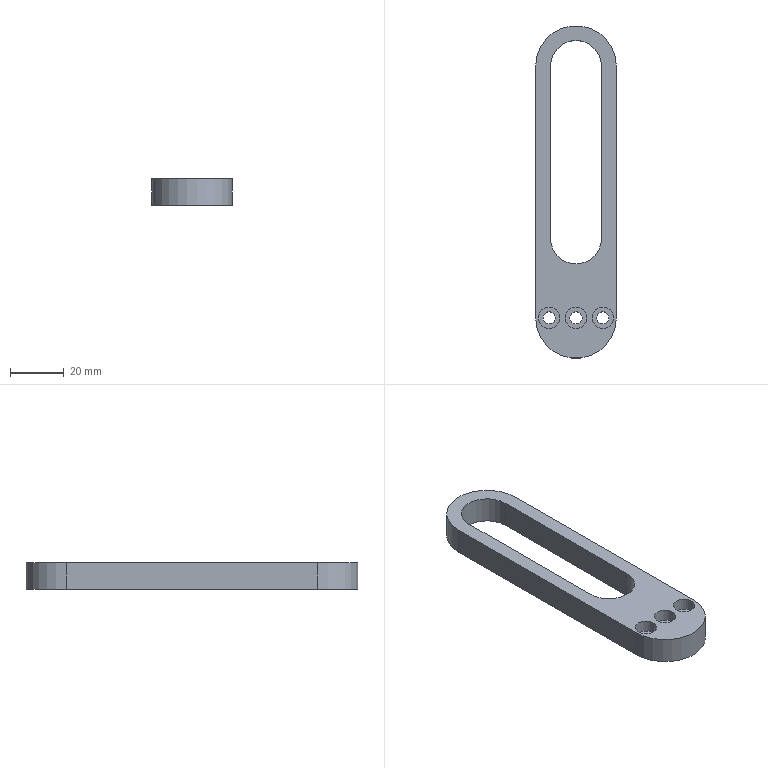Part | STEP file | 1 solid | 21 faces | box 30 x 123.5 x 10 mm | volume 18320 mm3 | cylinder 11 | plane 10 | commonest cylinder face diameters 4.5 x3 8 x3 19 x2 30 x2 28 x1
STEP:
#1=CARTESIAN_POINT('',(0.,0.,0.));
#2=DIRECTION('',(0.,0.,1.));
#3=DIRECTION('',(1.,0.,0.));
#4=AXIS2_PLACEMENT_3D('',#1,#2,#3);
#5=CARTESIAN_POINT('',(9.5,44.5,0.));
#6=VERTEX_POINT('',#5);
#7=CARTESIAN_POINT('',(9.5,108.5,0.));
#8=VERTEX_POINT('',#7);
#9=CARTESIAN_POINT('',(9.5,44.5,0.));
#10=DIRECTION('',(0.,1.,0.));
#11=VECTOR('',#10,1.);
#12=LINE('',#9,#11);
#13=CARTESIAN_POINT('',(9.5,44.5,0.));
#14=DIRECTION('',(-1.,0.,0.));
#15=DIRECTION('',(0.,0.,1.));
#16=AXIS2_PLACEMENT_3D('',#13,#14,#15);
#17=PLANE('',#16);
#18=CARTESIAN_POINT('',(0.,0.));
#19=DIRECTION('',(0.,1.));
#20=VECTOR('',#19,1.);
#21=LINE('',#18,#20);
#22=(GEOMETRIC_REPRESENTATION_CONTEXT(2)PARAMETRIC_REPRESENTATION_CONTEXT()REPRESENTATION_CONTEXT('',''));
#23=DEFINITIONAL_REPRESENTATION('',(#21),#22);
#24=PCURVE('',#17,#23);
#25=CARTESIAN_POINT('',(0.,0.,0.));
#26=DIRECTION('',(0.,0.,1.));
#27=DIRECTION('',(1.,0.,0.));
#28=AXIS2_PLACEMENT_3D('',#25,#26,#27);
#29=PLANE('',#28);
#30=CARTESIAN_POINT('',(9.5,44.5));
#31=DIRECTION('',(0.,1.));
#32=VECTOR('',#31,1.);
#33=LINE('',#30,#32);
#34=(GEOMETRIC_REPRESENTATION_CONTEXT(2)PARAMETRIC_REPRESENTATION_CONTEXT()REPRESENTATION_CONTEXT('',''));
#35=DEFINITIONAL_REPRESENTATION('',(#33),#34);
#36=PCURVE('',#29,#35);
#37=SURFACE_CURVE('',#12,(#24,#36),.PCURVE_S1.);
#38=EDGE_CURVE('',#6,#8,#37,.T.);
#39=ORIENTED_EDGE('',*,*,#38,.F.);
#40=CARTESIAN_POINT('',(9.5,44.5,10.));
#41=VERTEX_POINT('',#40);
#42=CARTESIAN_POINT('',(9.5,44.5,0.));
#43=DIRECTION('',(0.,0.,1.));
#44=VECTOR('',#43,1.);
#45=LINE('',#42,#44);
#46=CARTESIAN_POINT('',(0.,0.));
#47=DIRECTION('',(1.,0.));
#48=VECTOR('',#47,1.);
#49=LINE('',#46,#48);
#50=(GEOMETRIC_REPRESENTATION_CONTEXT(2)PARAMETRIC_REPRESENTATION_CONTEXT()REPRESENTATION_CONTEXT('',''));
#51=DEFINITIONAL_REPRESENTATION('',(#49),#50);
#52=PCURVE('',#17,#51);
#53=CARTESIAN_POINT('',(0.,44.5,0.));
#54=DIRECTION('',(0.,0.,1.));
#55=DIRECTION('',(-1.,0.,0.));
#56=AXIS2_PLACEMENT_3D('',#53,#54,#55);
#57=CYLINDRICAL_SURFACE('',#56,9.5);
#58=CARTESIAN_POINT('',(3.142,0.));
#59=DIRECTION('',(0.,1.));
#60=VECTOR('',#59,1.);
#61=LINE('',#58,#60);
#62=(GEOMETRIC_REPRESENTATION_CONTEXT(2)PARAMETRIC_REPRESENTATION_CONTEXT()REPRESENTATION_CONTEXT('',''));
#63=DEFINITIONAL_REPRESENTATION('',(#61),#62);
#64=PCURVE('',#57,#63);
#65=SURFACE_CURVE('',#45,(#52,#64),.PCURVE_S1.);
#66=EDGE_CURVE('',#6,#41,#65,.T.);
#67=ORIENTED_EDGE('',*,*,#66,.T.);
#68=CARTESIAN_POINT('',(9.5,108.5,10.));
#69=VERTEX_POINT('',#68);
#70=CARTESIAN_POINT('',(9.5,44.5,10.));
#71=DIRECTION('',(0.,1.,0.));
#72=VECTOR('',#71,1.);
#73=LINE('',#70,#72);
#74=CARTESIAN_POINT('',(10.,0.));
#75=DIRECTION('',(0.,1.));
#76=VECTOR('',#75,1.);
#77=LINE('',#74,#76);
#78=(GEOMETRIC_REPRESENTATION_CONTEXT(2)PARAMETRIC_REPRESENTATION_CONTEXT()REPRESENTATION_CONTEXT('',''));
#79=DEFINITIONAL_REPRESENTATION('',(#77),#78);
#80=PCURVE('',#17,#79);
#81=CARTESIAN_POINT('',(0.,0.,10.));
#82=DIRECTION('',(0.,0.,1.));
#83=DIRECTION('',(1.,0.,0.));
#84=AXIS2_PLACEMENT_3D('',#81,#82,#83);
#85=PLANE('',#84);
#86=CARTESIAN_POINT('',(9.5,44.5));
#87=DIRECTION('',(0.,1.));
#88=VECTOR('',#87,1.);
#89=LINE('',#86,#88);
#90=(GEOMETRIC_REPRESENTATION_CONTEXT(2)PARAMETRIC_REPRESENTATION_CONTEXT()REPRESENTATION_CONTEXT('',''));
#91=DEFINITIONAL_REPRESENTATION('',(#89),#90);
#92=PCURVE('',#85,#91);
#93=SURFACE_CURVE('',#73,(#80,#92),.PCURVE_S1.);
#94=EDGE_CURVE('',#41,#69,#93,.T.);
#95=ORIENTED_EDGE('',*,*,#94,.T.);
#96=CARTESIAN_POINT('',(9.5,108.5,0.));
#97=DIRECTION('',(0.,0.,1.));
#98=VECTOR('',#97,1.);
#99=LINE('',#96,#98);
#100=CARTESIAN_POINT('',(0.,64.));
#101=DIRECTION('',(1.,0.));
#102=VECTOR('',#101,1.);
#103=LINE('',#100,#102);
#104=(GEOMETRIC_REPRESENTATION_CONTEXT(2)PARAMETRIC_REPRESENTATION_CONTEXT()REPRESENTATION_CONTEXT('',''));
#105=DEFINITIONAL_REPRESENTATION('',(#103),#104);
#106=PCURVE('',#17,#105);
#107=CARTESIAN_POINT('',(0.,108.5,0.));
#108=DIRECTION('',(0.,0.,1.));
#109=DIRECTION('',(1.,0.,0.));
#110=AXIS2_PLACEMENT_3D('',#107,#108,#109);
#111=CYLINDRICAL_SURFACE('',#110,9.5);
#112=CARTESIAN_POINT('',(0.,0.));
#113=DIRECTION('',(0.,1.));
#114=VECTOR('',#113,1.);
#115=LINE('',#112,#114);
#116=(GEOMETRIC_REPRESENTATION_CONTEXT(2)PARAMETRIC_REPRESENTATION_CONTEXT()REPRESENTATION_CONTEXT('',''));
#117=DEFINITIONAL_REPRESENTATION('',(#115),#116);
#118=PCURVE('',#111,#117);
#119=SURFACE_CURVE('',#99,(#106,#118),.PCURVE_S1.);
#120=EDGE_CURVE('',#8,#69,#119,.T.);
#121=ORIENTED_EDGE('',*,*,#120,.F.);
#122=EDGE_LOOP('',(#39,#67,#95,#121));
#123=FACE_BOUND('',#122,.T.);
#124=ADVANCED_FACE('',(#123),#17,.T.);
#125=CARTESIAN_POINT('',(-15.,108.5,0.));
#126=VERTEX_POINT('',#125);
#127=CARTESIAN_POINT('',(-15.,15.,0.));
#128=VERTEX_POINT('',#127);
#129=CARTESIAN_POINT('',(-15.,108.5,0.));
#130=DIRECTION('',(0.,-1.,0.));
#131=VECTOR('',#130,1.);
#132=LINE('',#129,#131);
#133=CARTESIAN_POINT('',(-15.,108.5));
#134=DIRECTION('',(0.,-1.));
#135=VECTOR('',#134,1.);
#136=LINE('',#133,#135);
#137=(GEOMETRIC_REPRESENTATION_CONTEXT(2)PARAMETRIC_REPRESENTATION_CONTEXT()REPRESENTATION_CONTEXT('',''));
#138=DEFINITIONAL_REPRESENTATION('',(#136),#137);
#139=PCURVE('',#29,#138);
#140=CARTESIAN_POINT('',(-15.,15.,0.));
#141=DIRECTION('',(-1.,0.,0.));
#142=DIRECTION('',(0.,0.,1.));
#143=AXIS2_PLACEMENT_3D('',#140,#141,#142);
#144=PLANE('',#143);
#145=CARTESIAN_POINT('',(0.,93.5));
#146=DIRECTION('',(0.,-1.));
#147=VECTOR('',#146,1.);
#148=LINE('',#145,#147);
#149=(GEOMETRIC_REPRESENTATION_CONTEXT(2)PARAMETRIC_REPRESENTATION_CONTEXT()REPRESENTATION_CONTEXT('',''));
#150=DEFINITIONAL_REPRESENTATION('',(#148),#149);
#151=PCURVE('',#144,#150);
#152=SURFACE_CURVE('',#132,(#139,#151),.PCURVE_S1.);
#153=EDGE_CURVE('',#126,#128,#152,.T.);
#154=ORIENTED_EDGE('',*,*,#153,.F.);
#155=CARTESIAN_POINT('',(15.,108.5,0.));
#156=VERTEX_POINT('',#155);
#157=CARTESIAN_POINT('',(0.,108.5,0.));
#158=DIRECTION('',(0.,0.,1.));
#159=DIRECTION('',(1.,0.,0.));
#160=AXIS2_PLACEMENT_3D('',#157,#158,#159);
#161=CIRCLE('',#160,15.);
#162=CARTESIAN_POINT('',(0.,108.5));
#163=DIRECTION('',(1.,0.));
#164=AXIS2_PLACEMENT_2D('',#162,#163);
#165=CIRCLE('',#164,15.);
#166=(GEOMETRIC_REPRESENTATION_CONTEXT(2)PARAMETRIC_REPRESENTATION_CONTEXT()REPRESENTATION_CONTEXT('',''));
#167=DEFINITIONAL_REPRESENTATION('',(#165),#166);
#168=PCURVE('',#29,#167);
#169=CARTESIAN_POINT('',(0.,108.5,0.));
#170=DIRECTION('',(0.,0.,1.));
#171=DIRECTION('',(1.,0.,0.));
#172=AXIS2_PLACEMENT_3D('',#169,#170,#171);
#173=CYLINDRICAL_SURFACE('',#172,15.);
#174=CARTESIAN_POINT('',(0.,0.));
#175=DIRECTION('',(1.,0.));
#176=VECTOR('',#175,1.);
#177=LINE('',#174,#176);
#178=(GEOMETRIC_REPRESENTATION_CONTEXT(2)PARAMETRIC_REPRESENTATION_CONTEXT()REPRESENTATION_CONTEXT('',''));
#179=DEFINITIONAL_REPRESENTATION('',(#177),#178);
#180=PCURVE('',#173,#179);
#181=SURFACE_CURVE('',#161,(#168,#180),.PCURVE_S1.);
#182=EDGE_CURVE('',#156,#126,#181,.T.);
#183=ORIENTED_EDGE('',*,*,#182,.F.);
#184=CARTESIAN_POINT('',(15.,15.,0.));
#185=VERTEX_POINT('',#184);
#186=CARTESIAN_POINT('',(15.,15.,0.));
#187=DIRECTION('',(0.,1.,0.));
#188=VECTOR('',#187,1.);
#189=LINE('',#186,#188);
#190=CARTESIAN_POINT('',(15.,15.));
#191=DIRECTION('',(0.,1.));
#192=VECTOR('',#191,1.);
#193=LINE('',#190,#192);
#194=(GEOMETRIC_REPRESENTATION_CONTEXT(2)PARAMETRIC_REPRESENTATION_CONTEXT()REPRESENTATION_CONTEXT('',''));
#195=DEFINITIONAL_REPRESENTATION('',(#193),#194);
#196=PCURVE('',#29,#195);
#197=CARTESIAN_POINT('',(15.,108.5,0.));
#198=DIRECTION('',(1.,0.,0.));
#199=DIRECTION('',(0.,0.,-1.));
#200=AXIS2_PLACEMENT_3D('',#197,#198,#199);
#201=PLANE('',#200);
#202=CARTESIAN_POINT('',(0.,-93.5));
#203=DIRECTION('',(0.,1.));
#204=VECTOR('',#203,1.);
#205=LINE('',#202,#204);
#206=(GEOMETRIC_REPRESENTATION_CONTEXT(2)PARAMETRIC_REPRESENTATION_CONTEXT()REPRESENTATION_CONTEXT('',''));
#207=DEFINITIONAL_REPRESENTATION('',(#205),#206);
#208=PCURVE('',#201,#207);
#209=SURFACE_CURVE('',#189,(#196,#208),.PCURVE_S1.);
#210=EDGE_CURVE('',#185,#156,#209,.T.);
#211=ORIENTED_EDGE('',*,*,#210,.F.);
#212=CARTESIAN_POINT('',(0.,15.,0.));
#213=DIRECTION('',(0.,0.,1.));
#214=DIRECTION('',(1.,0.,0.));
#215=AXIS2_PLACEMENT_3D('',#212,#213,#214);
#216=CIRCLE('',#215,15.);
#217=CARTESIAN_POINT('',(0.,15.));
#218=DIRECTION('',(1.,0.));
#219=AXIS2_PLACEMENT_2D('',#217,#218);
#220=CIRCLE('',#219,15.);
#221=(GEOMETRIC_REPRESENTATION_CONTEXT(2)PARAMETRIC_REPRESENTATION_CONTEXT()REPRESENTATION_CONTEXT('',''));
#222=DEFINITIONAL_REPRESENTATION('',(#220),#221);
#223=PCURVE('',#29,#222);
#224=CARTESIAN_POINT('',(0.,15.,0.));
#225=DIRECTION('',(0.,0.,1.));
#226=DIRECTION('',(-1.,0.,0.));
#227=AXIS2_PLACEMENT_3D('',#224,#225,#226);
#228=CYLINDRICAL_SURFACE('',#227,15.);
#229=CARTESIAN_POINT('',(-3.142,0.));
#230=DIRECTION('',(1.,0.));
#231=VECTOR('',#230,1.);
#232=LINE('',#229,#231);
#233=(GEOMETRIC_REPRESENTATION_CONTEXT(2)PARAMETRIC_REPRESENTATION_CONTEXT()REPRESENTATION_CONTEXT('',''));
#234=DEFINITIONAL_REPRESENTATION('',(#232),#233);
#235=PCURVE('',#228,#234);
#236=SURFACE_CURVE('',#216,(#223,#235),.PCURVE_S1.);
#237=EDGE_CURVE('',#128,#185,#236,.T.);
#238=ORIENTED_EDGE('',*,*,#237,.F.);
#239=EDGE_LOOP('',(#154,#183,#211,#238));
#240=FACE_BOUND('',#239,.T.);
#241=CARTESIAN_POINT('',(-9.5,44.5,0.));
#242=VERTEX_POINT('',#241);
#243=CARTESIAN_POINT('',(0.,44.5,0.));
#244=DIRECTION('',(0.,0.,1.));
#245=DIRECTION('',(1.,0.,0.));
#246=AXIS2_PLACEMENT_3D('',#243,#244,#245);
#247=CIRCLE('',#246,9.5);
#248=CARTESIAN_POINT('',(0.,44.5));
#249=DIRECTION('',(1.,0.));
#250=AXIS2_PLACEMENT_2D('',#248,#249);
#251=CIRCLE('',#250,9.5);
#252=(GEOMETRIC_REPRESENTATION_CONTEXT(2)PARAMETRIC_REPRESENTATION_CONTEXT()REPRESENTATION_CONTEXT('',''));
#253=DEFINITIONAL_REPRESENTATION('',(#251),#252);
#254=PCURVE('',#29,#253);
#255=CARTESIAN_POINT('',(-3.142,0.));
#256=DIRECTION('',(1.,0.));
#257=VECTOR('',#256,1.);
#258=LINE('',#255,#257);
#259=(GEOMETRIC_REPRESENTATION_CONTEXT(2)PARAMETRIC_REPRESENTATION_CONTEXT()REPRESENTATION_CONTEXT('',''));
#260=DEFINITIONAL_REPRESENTATION('',(#258),#259);
#261=PCURVE('',#57,#260);
#262=SURFACE_CURVE('',#247,(#254,#261),.PCURVE_S1.);
#263=EDGE_CURVE('',#242,#6,#262,.T.);
#264=ORIENTED_EDGE('',*,*,#263,.T.);
#265=ORIENTED_EDGE('',*,*,#38,.T.);
#266=CARTESIAN_POINT('',(-9.5,108.5,0.));
#267=VERTEX_POINT('',#266);
#268=CARTESIAN_POINT('',(0.,108.5,0.));
#269=DIRECTION('',(0.,0.,1.));
#270=DIRECTION('',(1.,0.,0.));
#271=AXIS2_PLACEMENT_3D('',#268,#269,#270);
#272=CIRCLE('',#271,9.5);
#273=CARTESIAN_POINT('',(0.,108.5));
#274=DIRECTION('',(1.,0.));
#275=AXIS2_PLACEMENT_2D('',#273,#274);
#276=CIRCLE('',#275,9.5);
#277=(GEOMETRIC_REPRESENTATION_CONTEXT(2)PARAMETRIC_REPRESENTATION_CONTEXT()REPRESENTATION_CONTEXT('',''));
#278=DEFINITIONAL_REPRESENTATION('',(#276),#277);
#279=PCURVE('',#29,#278);
#280=CARTESIAN_POINT('',(0.,0.));
#281=DIRECTION('',(1.,0.));
#282=VECTOR('',#281,1.);
#283=LINE('',#280,#282);
#284=(GEOMETRIC_REPRESENTATION_CONTEXT(2)PARAMETRIC_REPRESENTATION_CONTEXT()REPRESENTATION_CONTEXT('',''));
#285=DEFINITIONAL_REPRESENTATION('',(#283),#284);
#286=PCURVE('',#111,#285);
#287=SURFACE_CURVE('',#272,(#279,#286),.PCURVE_S1.);
#288=EDGE_CURVE('',#8,#267,#287,.T.);
#289=ORIENTED_EDGE('',*,*,#288,.T.);
#290=CARTESIAN_POINT('',(-9.5,108.5,0.));
#291=DIRECTION('',(0.,-1.,0.));
#292=VECTOR('',#291,1.);
#293=LINE('',#290,#292);
#294=CARTESIAN_POINT('',(-9.5,108.5));
#295=DIRECTION('',(0.,-1.));
#296=VECTOR('',#295,1.);
#297=LINE('',#294,#296);
#298=(GEOMETRIC_REPRESENTATION_CONTEXT(2)PARAMETRIC_REPRESENTATION_CONTEXT()REPRESENTATION_CONTEXT('',''));
#299=DEFINITIONAL_REPRESENTATION('',(#297),#298);
#300=PCURVE('',#29,#299);
#301=CARTESIAN_POINT('',(-9.5,108.5,0.));
#302=DIRECTION('',(1.,0.,0.));
#303=DIRECTION('',(0.,0.,-1.));
#304=AXIS2_PLACEMENT_3D('',#301,#302,#303);
#305=PLANE('',#304);
#306=CARTESIAN_POINT('',(0.,0.));
#307=DIRECTION('',(0.,-1.));
#308=VECTOR('',#307,1.);
#309=LINE('',#306,#308);
#310=(GEOMETRIC_REPRESENTATION_CONTEXT(2)PARAMETRIC_REPRESENTATION_CONTEXT()REPRESENTATION_CONTEXT('',''));
#311=DEFINITIONAL_REPRESENTATION('',(#309),#310);
#312=PCURVE('',#305,#311);
#313=SURFACE_CURVE('',#293,(#300,#312),.PCURVE_S1.);
#314=EDGE_CURVE('',#267,#242,#313,.T.);
#315=ORIENTED_EDGE('',*,*,#314,.T.);
#316=EDGE_LOOP('',(#264,#265,#289,#315));
#317=FACE_BOUND('',#316,.T.);
#318=CARTESIAN_POINT('',(0.,29.,0.));
#319=VERTEX_POINT('',#318);
#320=CARTESIAN_POINT('',(0.,15.,0.));
#321=DIRECTION('',(0.,0.,1.));
#322=DIRECTION('',(1.,0.,0.));
#323=AXIS2_PLACEMENT_3D('',#320,#321,#322);
#324=CIRCLE('',#323,14.);
#325=CARTESIAN_POINT('',(0.,15.));
#326=DIRECTION('',(1.,0.));
#327=AXIS2_PLACEMENT_2D('',#325,#326);
#328=CIRCLE('',#327,14.);
#329=(GEOMETRIC_REPRESENTATION_CONTEXT(2)PARAMETRIC_REPRESENTATION_CONTEXT()REPRESENTATION_CONTEXT('',''));
#330=DEFINITIONAL_REPRESENTATION('',(#328),#329);
#331=PCURVE('',#29,#330);
#332=CARTESIAN_POINT('',(0.,15.,0.75));
#333=DIRECTION('',(0.,0.,1.));
#334=DIRECTION('',(0.,-1.,0.));
#335=AXIS2_PLACEMENT_3D('',#332,#333,#334);
#336=CYLINDRICAL_SURFACE('',#335,14.);
#337=CARTESIAN_POINT('',(1.571,-0.75));
#338=DIRECTION('',(1.,0.));
#339=VECTOR('',#338,1.);
#340=LINE('',#337,#339);
#341=(GEOMETRIC_REPRESENTATION_CONTEXT(2)PARAMETRIC_REPRESENTATION_CONTEXT()REPRESENTATION_CONTEXT('',''));
#342=DEFINITIONAL_REPRESENTATION('',(#340),#341);
#343=PCURVE('',#336,#342);
#344=SURFACE_CURVE('',#324,(#331,#343),.PCURVE_S1.);
#345=EDGE_CURVE('',#319,#319,#344,.T.);
#346=ORIENTED_EDGE('',*,*,#345,.T.);
#347=EDGE_LOOP('',(#346));
#348=FACE_BOUND('',#347,.T.);
#349=ADVANCED_FACE('',(#240,#317,#348),#29,.F.);
#350=ORIENTED_EDGE('',*,*,#66,.T.);
#351=CARTESIAN_POINT('',(-9.5,44.5,10.));
#352=VERTEX_POINT('',#351);
#353=CARTESIAN_POINT('',(0.,44.5,10.));
#354=DIRECTION('',(0.,0.,1.));
#355=DIRECTION('',(1.,0.,0.));
#356=AXIS2_PLACEMENT_3D('',#353,#354,#355);
#357=CIRCLE('',#356,9.5);
#358=CARTESIAN_POINT('',(-3.142,10.));
#359=DIRECTION('',(1.,0.));
#360=VECTOR('',#359,1.);
#361=LINE('',#358,#360);
#362=(GEOMETRIC_REPRESENTATION_CONTEXT(2)PARAMETRIC_REPRESENTATION_CONTEXT()REPRESENTATION_CONTEXT('',''));
#363=DEFINITIONAL_REPRESENTATION('',(#361),#362);
#364=PCURVE('',#57,#363);
#365=CARTESIAN_POINT('',(0.,44.5));
#366=DIRECTION('',(1.,0.));
#367=AXIS2_PLACEMENT_2D('',#365,#366);
#368=CIRCLE('',#367,9.5);
#369=(GEOMETRIC_REPRESENTATION_CONTEXT(2)PARAMETRIC_REPRESENTATION_CONTEXT()REPRESENTATION_CONTEXT('',''));
#370=DEFINITIONAL_REPRESENTATION('',(#368),#369);
#371=PCURVE('',#85,#370);
#372=SURFACE_CURVE('',#357,(#364,#371),.PCURVE_S1.);
#373=EDGE_CURVE('',#352,#41,#372,.T.);
#374=ORIENTED_EDGE('',*,*,#373,.F.);
#375=CARTESIAN_POINT('',(-9.5,44.5,0.));
#376=DIRECTION('',(0.,0.,1.));
#377=VECTOR('',#376,1.);
#378=LINE('',#375,#377);
#379=CARTESIAN_POINT('',(0.,0.));
#380=DIRECTION('',(0.,1.));
#381=VECTOR('',#380,1.);
#382=LINE('',#379,#381);
#383=(GEOMETRIC_REPRESENTATION_CONTEXT(2)PARAMETRIC_REPRESENTATION_CONTEXT()REPRESENTATION_CONTEXT('',''));
#384=DEFINITIONAL_REPRESENTATION('',(#382),#383);
#385=PCURVE('',#57,#384);
#386=CARTESIAN_POINT('',(0.,-64.));
#387=DIRECTION('',(-1.,0.));
#388=VECTOR('',#387,1.);
#389=LINE('',#386,#388);
#390=(GEOMETRIC_REPRESENTATION_CONTEXT(2)PARAMETRIC_REPRESENTATION_CONTEXT()REPRESENTATION_CONTEXT('',''));
#391=DEFINITIONAL_REPRESENTATION('',(#389),#390);
#392=PCURVE('',#305,#391);
#393=SURFACE_CURVE('',#378,(#385,#392),.PCURVE_S1.);
#394=EDGE_CURVE('',#242,#352,#393,.T.);
#395=ORIENTED_EDGE('',*,*,#394,.F.);
#396=ORIENTED_EDGE('',*,*,#263,.T.);
#397=EDGE_LOOP('',(#350,#374,#395,#396));
#398=FACE_BOUND('',#397,.F.);
#399=ADVANCED_FACE('',(#398),#57,.F.);
#400=CARTESIAN_POINT('',(-15.,15.,10.));
#401=VERTEX_POINT('',#400);
#402=CARTESIAN_POINT('',(15.,15.,10.));
#403=VERTEX_POINT('',#402);
#404=CARTESIAN_POINT('',(0.,15.,10.));
#405=DIRECTION('',(0.,0.,1.));
#406=DIRECTION('',(1.,0.,0.));
#407=AXIS2_PLACEMENT_3D('',#404,#405,#406);
#408=CIRCLE('',#407,15.);
#409=CARTESIAN_POINT('',(0.,15.));
#410=DIRECTION('',(1.,0.));
#411=AXIS2_PLACEMENT_2D('',#409,#410);
#412=CIRCLE('',#411,15.);
#413=(GEOMETRIC_REPRESENTATION_CONTEXT(2)PARAMETRIC_REPRESENTATION_CONTEXT()REPRESENTATION_CONTEXT('',''));
#414=DEFINITIONAL_REPRESENTATION('',(#412),#413);
#415=PCURVE('',#85,#414);
#416=CARTESIAN_POINT('',(-3.142,10.));
#417=DIRECTION('',(1.,0.));
#418=VECTOR('',#417,1.);
#419=LINE('',#416,#418);
#420=(GEOMETRIC_REPRESENTATION_CONTEXT(2)PARAMETRIC_REPRESENTATION_CONTEXT()REPRESENTATION_CONTEXT('',''));
#421=DEFINITIONAL_REPRESENTATION('',(#419),#420);
#422=PCURVE('',#228,#421);
#423=SURFACE_CURVE('',#408,(#415,#422),.PCURVE_S1.);
#424=EDGE_CURVE('',#401,#403,#423,.T.);
#425=ORIENTED_EDGE('',*,*,#424,.T.);
#426=CARTESIAN_POINT('',(15.,108.5,10.));
#427=VERTEX_POINT('',#426);
#428=CARTESIAN_POINT('',(15.,15.,10.));
#429=DIRECTION('',(0.,1.,0.));
#430=VECTOR('',#429,1.);
#431=LINE('',#428,#430);
#432=CARTESIAN_POINT('',(15.,15.));
#433=DIRECTION('',(0.,1.));
#434=VECTOR('',#433,1.);
#435=LINE('',#432,#434);
#436=(GEOMETRIC_REPRESENTATION_CONTEXT(2)PARAMETRIC_REPRESENTATION_CONTEXT()REPRESENTATION_CONTEXT('',''));
#437=DEFINITIONAL_REPRESENTATION('',(#435),#436);
#438=PCURVE('',#85,#437);
#439=CARTESIAN_POINT('',(-10.,-93.5));
#440=DIRECTION('',(0.,1.));
#441=VECTOR('',#440,1.);
#442=LINE('',#439,#441);
#443=(GEOMETRIC_REPRESENTATION_CONTEXT(2)PARAMETRIC_REPRESENTATION_CONTEXT()REPRESENTATION_CONTEXT('',''));
#444=DEFINITIONAL_REPRESENTATION('',(#442),#443);
#445=PCURVE('',#201,#444);
#446=SURFACE_CURVE('',#431,(#438,#445),.PCURVE_S1.);
#447=EDGE_CURVE('',#403,#427,#446,.T.);
#448=ORIENTED_EDGE('',*,*,#447,.T.);
#449=CARTESIAN_POINT('',(-15.,108.5,10.));
#450=VERTEX_POINT('',#449);
#451=CARTESIAN_POINT('',(0.,108.5,10.));
#452=DIRECTION('',(0.,0.,1.));
#453=DIRECTION('',(1.,0.,0.));
#454=AXIS2_PLACEMENT_3D('',#451,#452,#453);
#455=CIRCLE('',#454,15.);
#456=CARTESIAN_POINT('',(0.,108.5));
#457=DIRECTION('',(1.,0.));
#458=AXIS2_PLACEMENT_2D('',#456,#457);
#459=CIRCLE('',#458,15.);
#460=(GEOMETRIC_REPRESENTATION_CONTEXT(2)PARAMETRIC_REPRESENTATION_CONTEXT()REPRESENTATION_CONTEXT('',''));
#461=DEFINITIONAL_REPRESENTATION('',(#459),#460);
#462=PCURVE('',#85,#461);
#463=CARTESIAN_POINT('',(0.,10.));
#464=DIRECTION('',(1.,0.));
#465=VECTOR('',#464,1.);
#466=LINE('',#463,#465);
#467=(GEOMETRIC_REPRESENTATION_CONTEXT(2)PARAMETRIC_REPRESENTATION_CONTEXT()REPRESENTATION_CONTEXT('',''));
#468=DEFINITIONAL_REPRESENTATION('',(#466),#467);
#469=PCURVE('',#173,#468);
#470=SURFACE_CURVE('',#455,(#462,#469),.PCURVE_S1.);
#471=EDGE_CURVE('',#427,#450,#470,.T.);
#472=ORIENTED_EDGE('',*,*,#471,.T.);
#473=CARTESIAN_POINT('',(-15.,108.5,10.));
#474=DIRECTION('',(0.,-1.,0.));
#475=VECTOR('',#474,1.);
#476=LINE('',#473,#475);
#477=CARTESIAN_POINT('',(-15.,108.5));
#478=DIRECTION('',(0.,-1.));
#479=VECTOR('',#478,1.);
#480=LINE('',#477,#479);
#481=(GEOMETRIC_REPRESENTATION_CONTEXT(2)PARAMETRIC_REPRESENTATION_CONTEXT()REPRESENTATION_CONTEXT('',''));
#482=DEFINITIONAL_REPRESENTATION('',(#480),#481);
#483=PCURVE('',#85,#482);
#484=CARTESIAN_POINT('',(10.,93.5));
#485=DIRECTION('',(0.,-1.));
#486=VECTOR('',#485,1.);
#487=LINE('',#484,#486);
#488=(GEOMETRIC_REPRESENTATION_CONTEXT(2)PARAMETRIC_REPRESENTATION_CONTEXT()REPRESENTATION_CONTEXT('',''));
#489=DEFINITIONAL_REPRESENTATION('',(#487),#488);
#490=PCURVE('',#144,#489);
#491=SURFACE_CURVE('',#476,(#483,#490),.PCURVE_S1.);
#492=EDGE_CURVE('',#450,#401,#491,.T.);
#493=ORIENTED_EDGE('',*,*,#492,.T.);
#494=EDGE_LOOP('',(#425,#448,#472,#493));
#495=FACE_BOUND('',#494,.T.);
#496=CARTESIAN_POINT('',(-9.5,108.5,10.));
#497=VERTEX_POINT('',#496);
#498=CARTESIAN_POINT('',(-9.5,108.5,10.));
#499=DIRECTION('',(0.,-1.,0.));
#500=VECTOR('',#499,1.);
#501=LINE('',#498,#500);
#502=CARTESIAN_POINT('',(-9.5,108.5));
#503=DIRECTION('',(0.,-1.));
#504=VECTOR('',#503,1.);
#505=LINE('',#502,#504);
#506=(GEOMETRIC_REPRESENTATION_CONTEXT(2)PARAMETRIC_REPRESENTATION_CONTEXT()REPRESENTATION_CONTEXT('',''));
#507=DEFINITIONAL_REPRESENTATION('',(#505),#506);
#508=PCURVE('',#85,#507);
#509=CARTESIAN_POINT('',(-10.,0.));
#510=DIRECTION('',(0.,-1.));
#511=VECTOR('',#510,1.);
#512=LINE('',#509,#511);
#513=(GEOMETRIC_REPRESENTATION_CONTEXT(2)PARAMETRIC_REPRESENTATION_CONTEXT()REPRESENTATION_CONTEXT('',''));
#514=DEFINITIONAL_REPRESENTATION('',(#512),#513);
#515=PCURVE('',#305,#514);
#516=SURFACE_CURVE('',#501,(#508,#515),.PCURVE_S1.);
#517=EDGE_CURVE('',#497,#352,#516,.T.);
#518=ORIENTED_EDGE('',*,*,#517,.F.);
#519=CARTESIAN_POINT('',(0.,108.5,10.));
#520=DIRECTION('',(0.,0.,1.));
#521=DIRECTION('',(1.,0.,0.));
#522=AXIS2_PLACEMENT_3D('',#519,#520,#521);
#523=CIRCLE('',#522,9.5);
#524=CARTESIAN_POINT('',(0.,108.5));
#525=DIRECTION('',(1.,0.));
#526=AXIS2_PLACEMENT_2D('',#524,#525);
#527=CIRCLE('',#526,9.5);
#528=(GEOMETRIC_REPRESENTATION_CONTEXT(2)PARAMETRIC_REPRESENTATION_CONTEXT()REPRESENTATION_CONTEXT('',''));
#529=DEFINITIONAL_REPRESENTATION('',(#527),#528);
#530=PCURVE('',#85,#529);
#531=CARTESIAN_POINT('',(0.,10.));
#532=DIRECTION('',(1.,0.));
#533=VECTOR('',#532,1.);
#534=LINE('',#531,#533);
#535=(GEOMETRIC_REPRESENTATION_CONTEXT(2)PARAMETRIC_REPRESENTATION_CONTEXT()REPRESENTATION_CONTEXT('',''));
#536=DEFINITIONAL_REPRESENTATION('',(#534),#535);
#537=PCURVE('',#111,#536);
#538=SURFACE_CURVE('',#523,(#530,#537),.PCURVE_S1.);
#539=EDGE_CURVE('',#69,#497,#538,.T.);
#540=ORIENTED_EDGE('',*,*,#539,.F.);
#541=ORIENTED_EDGE('',*,*,#94,.F.);
#542=ORIENTED_EDGE('',*,*,#373,.F.);
#543=EDGE_LOOP('',(#518,#540,#541,#542));
#544=FACE_BOUND('',#543,.T.);
#545=CARTESIAN_POINT('',(10.,11.,10.));
#546=VERTEX_POINT('',#545);
#547=CARTESIAN_POINT('',(10.,15.,10.));
#548=DIRECTION('',(0.,0.,1.));
#549=DIRECTION('',(1.,0.,0.));
#550=AXIS2_PLACEMENT_3D('',#547,#548,#549);
#551=CIRCLE('',#550,4.);
#552=CARTESIAN_POINT('',(10.,15.));
#553=DIRECTION('',(1.,0.));
#554=AXIS2_PLACEMENT_2D('',#552,#553);
#555=CIRCLE('',#554,4.);
#556=(GEOMETRIC_REPRESENTATION_CONTEXT(2)PARAMETRIC_REPRESENTATION_CONTEXT()REPRESENTATION_CONTEXT('',''));
#557=DEFINITIONAL_REPRESENTATION('',(#555),#556);
#558=PCURVE('',#85,#557);
#559=CARTESIAN_POINT('',(10.,15.,7.7));
#560=DIRECTION('',(0.,0.,1.));
#561=DIRECTION('',(0.,-1.,0.));
#562=AXIS2_PLACEMENT_3D('',#559,#560,#561);
#563=CYLINDRICAL_SURFACE('',#562,4.);
#564=CARTESIAN_POINT('',(-4.712,2.3));
#565=DIRECTION('',(1.,0.));
#566=VECTOR('',#565,1.);
#567=LINE('',#564,#566);
#568=(GEOMETRIC_REPRESENTATION_CONTEXT(2)PARAMETRIC_REPRESENTATION_CONTEXT()REPRESENTATION_CONTEXT('',''));
#569=DEFINITIONAL_REPRESENTATION('',(#567),#568);
#570=PCURVE('',#563,#569);
#571=SURFACE_CURVE('',#551,(#558,#570),.PCURVE_S1.);
#572=EDGE_CURVE('',#546,#546,#571,.T.);
#573=ORIENTED_EDGE('',*,*,#572,.F.);
#574=EDGE_LOOP('',(#573));
#575=FACE_BOUND('',#574,.T.);
#576=CARTESIAN_POINT('',(-10.,11.,10.));
#577=VERTEX_POINT('',#576);
#578=CARTESIAN_POINT('',(-10.,15.,10.));
#579=DIRECTION('',(0.,0.,1.));
#580=DIRECTION('',(1.,0.,0.));
#581=AXIS2_PLACEMENT_3D('',#578,#579,#580);
#582=CIRCLE('',#581,4.);
#583=CARTESIAN_POINT('',(-10.,15.));
#584=DIRECTION('',(1.,0.));
#585=AXIS2_PLACEMENT_2D('',#583,#584);
#586=CIRCLE('',#585,4.);
#587=(GEOMETRIC_REPRESENTATION_CONTEXT(2)PARAMETRIC_REPRESENTATION_CONTEXT()REPRESENTATION_CONTEXT('',''));
#588=DEFINITIONAL_REPRESENTATION('',(#586),#587);
#589=PCURVE('',#85,#588);
#590=CARTESIAN_POINT('',(-10.,15.,7.7));
#591=DIRECTION('',(0.,0.,1.));
#592=DIRECTION('',(0.,-1.,0.));
#593=AXIS2_PLACEMENT_3D('',#590,#591,#592);
#594=CYLINDRICAL_SURFACE('',#593,4.);
#595=CARTESIAN_POINT('',(-4.712,2.3));
#596=DIRECTION('',(1.,0.));
#597=VECTOR('',#596,1.);
#598=LINE('',#595,#597);
#599=(GEOMETRIC_REPRESENTATION_CONTEXT(2)PARAMETRIC_REPRESENTATION_CONTEXT()REPRESENTATION_CONTEXT('',''));
#600=DEFINITIONAL_REPRESENTATION('',(#598),#599);
#601=PCURVE('',#594,#600);
#602=SURFACE_CURVE('',#582,(#589,#601),.PCURVE_S1.);
#603=EDGE_CURVE('',#577,#577,#602,.T.);
#604=ORIENTED_EDGE('',*,*,#603,.F.);
#605=EDGE_LOOP('',(#604));
#606=FACE_BOUND('',#605,.T.);
#607=CARTESIAN_POINT('',(0.,11.,10.));
#608=VERTEX_POINT('',#607);
#609=CARTESIAN_POINT('',(0.,15.,10.));
#610=DIRECTION('',(0.,0.,1.));
#611=DIRECTION('',(1.,0.,0.));
#612=AXIS2_PLACEMENT_3D('',#609,#610,#611);
#613=CIRCLE('',#612,4.);
#614=CARTESIAN_POINT('',(0.,15.));
#615=DIRECTION('',(1.,0.));
#616=AXIS2_PLACEMENT_2D('',#614,#615);
#617=CIRCLE('',#616,4.);
#618=(GEOMETRIC_REPRESENTATION_CONTEXT(2)PARAMETRIC_REPRESENTATION_CONTEXT()REPRESENTATION_CONTEXT('',''));
#619=DEFINITIONAL_REPRESENTATION('',(#617),#618);
#620=PCURVE('',#85,#619);
#621=CARTESIAN_POINT('',(0.,15.,7.7));
#622=DIRECTION('',(0.,0.,1.));
#623=DIRECTION('',(0.,-1.,0.));
#624=AXIS2_PLACEMENT_3D('',#621,#622,#623);
#625=CYLINDRICAL_SURFACE('',#624,4.);
#626=CARTESIAN_POINT('',(-4.712,2.3));
#627=DIRECTION('',(1.,0.));
#628=VECTOR('',#627,1.);
#629=LINE('',#626,#628);
#630=(GEOMETRIC_REPRESENTATION_CONTEXT(2)PARAMETRIC_REPRESENTATION_CONTEXT()REPRESENTATION_CONTEXT('',''));
#631=DEFINITIONAL_REPRESENTATION('',(#629),#630);
#632=PCURVE('',#625,#631);
#633=SURFACE_CURVE('',#613,(#620,#632),.PCURVE_S1.);
#634=EDGE_CURVE('',#608,#608,#633,.T.);
#635=ORIENTED_EDGE('',*,*,#634,.F.);
#636=EDGE_LOOP('',(#635));
#637=FACE_BOUND('',#636,.T.);
#638=ADVANCED_FACE('',(#495,#544,#575,#606,#637),#85,.T.);
#639=CARTESIAN_POINT('',(-9.5,108.5,0.));
#640=DIRECTION('',(0.,0.,1.));
#641=VECTOR('',#640,1.);
#642=LINE('',#639,#641);
#643=CARTESIAN_POINT('',(3.142,0.));
#644=DIRECTION('',(0.,1.));
#645=VECTOR('',#644,1.);
#646=LINE('',#643,#645);
#647=(GEOMETRIC_REPRESENTATION_CONTEXT(2)PARAMETRIC_REPRESENTATION_CONTEXT()REPRESENTATION_CONTEXT('',''));
#648=DEFINITIONAL_REPRESENTATION('',(#646),#647);
#649=PCURVE('',#111,#648);
#650=CARTESIAN_POINT('',(0.,0.));
#651=DIRECTION('',(-1.,0.));
#652=VECTOR('',#651,1.);
#653=LINE('',#650,#652);
#654=(GEOMETRIC_REPRESENTATION_CONTEXT(2)PARAMETRIC_REPRESENTATION_CONTEXT()REPRESENTATION_CONTEXT('',''));
#655=DEFINITIONAL_REPRESENTATION('',(#653),#654);
#656=PCURVE('',#305,#655);
#657=SURFACE_CURVE('',#642,(#649,#656),.PCURVE_S1.);
#658=EDGE_CURVE('',#267,#497,#657,.T.);
#659=ORIENTED_EDGE('',*,*,#658,.T.);
#660=ORIENTED_EDGE('',*,*,#539,.F.);
#661=ORIENTED_EDGE('',*,*,#120,.F.);
#662=ORIENTED_EDGE('',*,*,#288,.T.);
#663=EDGE_LOOP('',(#659,#660,#661,#662));
#664=FACE_BOUND('',#663,.F.);
#665=ADVANCED_FACE('',(#664),#111,.F.);
#666=ORIENTED_EDGE('',*,*,#153,.T.);
#667=CARTESIAN_POINT('',(-15.,15.,0.));
#668=DIRECTION('',(0.,0.,1.));
#669=VECTOR('',#668,1.);
#670=LINE('',#667,#669);
#671=CARTESIAN_POINT('',(0.,0.));
#672=DIRECTION('',(1.,0.));
#673=VECTOR('',#672,1.);
#674=LINE('',#671,#673);
#675=(GEOMETRIC_REPRESENTATION_CONTEXT(2)PARAMETRIC_REPRESENTATION_CONTEXT()REPRESENTATION_CONTEXT('',''));
#676=DEFINITIONAL_REPRESENTATION('',(#674),#675);
#677=PCURVE('',#144,#676);
#678=CARTESIAN_POINT('',(0.,0.));
#679=DIRECTION('',(0.,1.));
#680=VECTOR('',#679,1.);
#681=LINE('',#678,#680);
#682=(GEOMETRIC_REPRESENTATION_CONTEXT(2)PARAMETRIC_REPRESENTATION_CONTEXT()REPRESENTATION_CONTEXT('',''));
#683=DEFINITIONAL_REPRESENTATION('',(#681),#682);
#684=PCURVE('',#228,#683);
#685=SURFACE_CURVE('',#670,(#677,#684),.PCURVE_S1.);
#686=EDGE_CURVE('',#128,#401,#685,.T.);
#687=ORIENTED_EDGE('',*,*,#686,.T.);
#688=ORIENTED_EDGE('',*,*,#492,.F.);
#689=CARTESIAN_POINT('',(-15.,108.5,0.));
#690=DIRECTION('',(0.,0.,1.));
#691=VECTOR('',#690,1.);
#692=LINE('',#689,#691);
#693=CARTESIAN_POINT('',(0.,93.5));
#694=DIRECTION('',(1.,0.));
#695=VECTOR('',#694,1.);
#696=LINE('',#693,#695);
#697=(GEOMETRIC_REPRESENTATION_CONTEXT(2)PARAMETRIC_REPRESENTATION_CONTEXT()REPRESENTATION_CONTEXT('',''));
#698=DEFINITIONAL_REPRESENTATION('',(#696),#697);
#699=PCURVE('',#144,#698);
#700=CARTESIAN_POINT('',(3.142,0.));
#701=DIRECTION('',(0.,1.));
#702=VECTOR('',#701,1.);
#703=LINE('',#700,#702);
#704=(GEOMETRIC_REPRESENTATION_CONTEXT(2)PARAMETRIC_REPRESENTATION_CONTEXT()REPRESENTATION_CONTEXT('',''));
#705=DEFINITIONAL_REPRESENTATION('',(#703),#704);
#706=PCURVE('',#173,#705);
#707=SURFACE_CURVE('',#692,(#699,#706),.PCURVE_S1.);
#708=EDGE_CURVE('',#126,#450,#707,.T.);
#709=ORIENTED_EDGE('',*,*,#708,.F.);
#710=EDGE_LOOP('',(#666,#687,#688,#709));
#711=FACE_BOUND('',#710,.T.);
#712=ADVANCED_FACE('',(#711),#144,.T.);
#713=ORIENTED_EDGE('',*,*,#182,.T.);
#714=ORIENTED_EDGE('',*,*,#708,.T.);
#715=ORIENTED_EDGE('',*,*,#471,.F.);
#716=CARTESIAN_POINT('',(15.,108.5,0.));
#717=DIRECTION('',(0.,0.,1.));
#718=VECTOR('',#717,1.);
#719=LINE('',#716,#718);
#720=CARTESIAN_POINT('',(0.,0.));
#721=DIRECTION('',(0.,1.));
#722=VECTOR('',#721,1.);
#723=LINE('',#720,#722);
#724=(GEOMETRIC_REPRESENTATION_CONTEXT(2)PARAMETRIC_REPRESENTATION_CONTEXT()REPRESENTATION_CONTEXT('',''));
#725=DEFINITIONAL_REPRESENTATION('',(#723),#724);
#726=PCURVE('',#173,#725);
#727=CARTESIAN_POINT('',(0.,0.));
#728=DIRECTION('',(-1.,0.));
#729=VECTOR('',#728,1.);
#730=LINE('',#727,#729);
#731=(GEOMETRIC_REPRESENTATION_CONTEXT(2)PARAMETRIC_REPRESENTATION_CONTEXT()REPRESENTATION_CONTEXT('',''));
#732=DEFINITIONAL_REPRESENTATION('',(#730),#731);
#733=PCURVE('',#201,#732);
#734=SURFACE_CURVE('',#719,(#726,#733),.PCURVE_S1.);
#735=EDGE_CURVE('',#156,#427,#734,.T.);
#736=ORIENTED_EDGE('',*,*,#735,.F.);
#737=EDGE_LOOP('',(#713,#714,#715,#736));
#738=FACE_BOUND('',#737,.T.);
#739=ADVANCED_FACE('',(#738),#173,.T.);
#740=ORIENTED_EDGE('',*,*,#210,.T.);
#741=ORIENTED_EDGE('',*,*,#735,.T.);
#742=ORIENTED_EDGE('',*,*,#447,.F.);
#743=CARTESIAN_POINT('',(15.,15.,0.));
#744=DIRECTION('',(0.,0.,1.));
#745=VECTOR('',#744,1.);
#746=LINE('',#743,#745);
#747=CARTESIAN_POINT('',(0.,-93.5));
#748=DIRECTION('',(-1.,0.));
#749=VECTOR('',#748,1.);
#750=LINE('',#747,#749);
#751=(GEOMETRIC_REPRESENTATION_CONTEXT(2)PARAMETRIC_REPRESENTATION_CONTEXT()REPRESENTATION_CONTEXT('',''));
#752=DEFINITIONAL_REPRESENTATION('',(#750),#751);
#753=PCURVE('',#201,#752);
#754=CARTESIAN_POINT('',(3.142,0.));
#755=DIRECTION('',(0.,1.));
#756=VECTOR('',#755,1.);
#757=LINE('',#754,#756);
#758=(GEOMETRIC_REPRESENTATION_CONTEXT(2)PARAMETRIC_REPRESENTATION_CONTEXT()REPRESENTATION_CONTEXT('',''));
#759=DEFINITIONAL_REPRESENTATION('',(#757),#758);
#760=PCURVE('',#228,#759);
#761=SURFACE_CURVE('',#746,(#753,#760),.PCURVE_S1.);
#762=EDGE_CURVE('',#185,#403,#761,.T.);
#763=ORIENTED_EDGE('',*,*,#762,.F.);
#764=EDGE_LOOP('',(#740,#741,#742,#763));
#765=FACE_BOUND('',#764,.T.);
#766=ADVANCED_FACE('',(#765),#201,.T.);
#767=ORIENTED_EDGE('',*,*,#237,.T.);
#768=ORIENTED_EDGE('',*,*,#762,.T.);
#769=ORIENTED_EDGE('',*,*,#424,.F.);
#770=ORIENTED_EDGE('',*,*,#686,.F.);
#771=EDGE_LOOP('',(#767,#768,#769,#770));
#772=FACE_BOUND('',#771,.T.);
#773=ADVANCED_FACE('',(#772),#228,.T.);
#774=ORIENTED_EDGE('',*,*,#314,.F.);
#775=ORIENTED_EDGE('',*,*,#658,.T.);
#776=ORIENTED_EDGE('',*,*,#517,.T.);
#777=ORIENTED_EDGE('',*,*,#394,.F.);
#778=EDGE_LOOP('',(#774,#775,#776,#777));
#779=FACE_BOUND('',#778,.T.);
#780=ADVANCED_FACE('',(#779),#305,.T.);
#781=ORIENTED_EDGE('',*,*,#345,.T.);
#782=CARTESIAN_POINT('',(0.,29.,1.5));
#783=VERTEX_POINT('',#782);
#784=CARTESIAN_POINT('',(0.,29.,0.));
#785=CARTESIAN_POINT('',(0.,29.,1.5));
#786=B_SPLINE_CURVE_WITH_KNOTS('',1,(#784,#785),.UNSPECIFIED.,.F.,.F.,(2,2),(-0.75,0.75),.PIECEWISE_BEZIER_KNOTS.);
#787=CARTESIAN_POINT('',(9.425,0.));
#788=DIRECTION('',(0.,1.));
#789=VECTOR('',#788,1.);
#790=LINE('',#787,#789);
#791=(GEOMETRIC_REPRESENTATION_CONTEXT(2)PARAMETRIC_REPRESENTATION_CONTEXT()REPRESENTATION_CONTEXT('',''));
#792=DEFINITIONAL_REPRESENTATION('',(#790),#791);
#793=PCURVE('',#336,#792);
#794=CARTESIAN_POINT('',(3.142,0.));
#795=DIRECTION('',(0.,1.));
#796=VECTOR('',#795,1.);
#797=LINE('',#794,#796);
#798=(GEOMETRIC_REPRESENTATION_CONTEXT(2)PARAMETRIC_REPRESENTATION_CONTEXT()REPRESENTATION_CONTEXT('',''));
#799=DEFINITIONAL_REPRESENTATION('',(#797),#798);
#800=PCURVE('',#336,#799);
#801=SEAM_CURVE('',#786,(#793,#800),.PCURVE_S1.);
#802=EDGE_CURVE('',#319,#783,#801,.T.);
#803=ORIENTED_EDGE('',*,*,#802,.T.);
#804=CARTESIAN_POINT('',(0.,15.,1.5));
#805=DIRECTION('',(0.,0.,1.));
#806=DIRECTION('',(1.,0.,0.));
#807=AXIS2_PLACEMENT_3D('',#804,#805,#806);
#808=CIRCLE('',#807,14.);
#809=CARTESIAN_POINT('',(1.571,0.75));
#810=DIRECTION('',(1.,0.));
#811=VECTOR('',#810,1.);
#812=LINE('',#809,#811);
#813=(GEOMETRIC_REPRESENTATION_CONTEXT(2)PARAMETRIC_REPRESENTATION_CONTEXT()REPRESENTATION_CONTEXT('',''));
#814=DEFINITIONAL_REPRESENTATION('',(#812),#813);
#815=PCURVE('',#336,#814);
#816=CARTESIAN_POINT('',(0.,22.,1.5));
#817=DIRECTION('',(0.,0.,-1.));
#818=DIRECTION('',(-1.,0.,0.));
#819=AXIS2_PLACEMENT_3D('',#816,#817,#818);
#820=PLANE('',#819);
#821=CARTESIAN_POINT('',(-14.,-7.));
#822=CARTESIAN_POINT('',(-14.,17.249));
#823=CARTESIAN_POINT('',(7.,5.124));
#824=CARTESIAN_POINT('',(28.,-7.));
#825=CARTESIAN_POINT('',(7.,-19.124));
#826=CARTESIAN_POINT('',(-14.,-31.249));
#827=CARTESIAN_POINT('',(-14.,-7.));
#828=(BOUNDED_CURVE()B_SPLINE_CURVE(2,(#821,#822,#823,#824,#825,#826,#827),.UNSPECIFIED.,.T.,.F.)B_SPLINE_CURVE_WITH_KNOTS((1,2,2,2,2,1),(-2.094,0.,2.094,4.189,6.283,8.378),.UNSPECIFIED.)CURVE()GEOMETRIC_REPRESENTATION_ITEM()RATIONAL_B_SPLINE_CURVE((1.,0.5,1.,0.5,1.,0.5,1.))REPRESENTATION_ITEM(''));
#829=(GEOMETRIC_REPRESENTATION_CONTEXT(2)PARAMETRIC_REPRESENTATION_CONTEXT()REPRESENTATION_CONTEXT('',''));
#830=DEFINITIONAL_REPRESENTATION('',(#828),#829);
#831=PCURVE('',#820,#830);
#832=SURFACE_CURVE('',#808,(#815,#831),.PCURVE_S1.);
#833=EDGE_CURVE('',#783,#783,#832,.T.);
#834=ORIENTED_EDGE('',*,*,#833,.F.);
#835=ORIENTED_EDGE('',*,*,#802,.F.);
#836=EDGE_LOOP('',(#781,#803,#834,#835));
#837=FACE_BOUND('',#836,.F.);
#838=ADVANCED_FACE('',(#837),#336,.F.);
#839=ORIENTED_EDGE('',*,*,#572,.F.);
#840=CARTESIAN_POINT('',(10.,11.,5.4));
#841=VERTEX_POINT('',#840);
#842=CARTESIAN_POINT('',(10.,11.,5.4));
#843=CARTESIAN_POINT('',(10.,11.,10.));
#844=B_SPLINE_CURVE_WITH_KNOTS('',1,(#842,#843),.UNSPECIFIED.,.F.,.F.,(2,2),(-2.3,2.3),.PIECEWISE_BEZIER_KNOTS.);
#845=CARTESIAN_POINT('',(0.,0.));
#846=DIRECTION('',(0.,1.));
#847=VECTOR('',#846,1.);
#848=LINE('',#845,#847);
#849=(GEOMETRIC_REPRESENTATION_CONTEXT(2)PARAMETRIC_REPRESENTATION_CONTEXT()REPRESENTATION_CONTEXT('',''));
#850=DEFINITIONAL_REPRESENTATION('',(#848),#849);
#851=PCURVE('',#563,#850);
#852=CARTESIAN_POINT('',(6.283,0.));
#853=DIRECTION('',(0.,1.));
#854=VECTOR('',#853,1.);
#855=LINE('',#852,#854);
#856=(GEOMETRIC_REPRESENTATION_CONTEXT(2)PARAMETRIC_REPRESENTATION_CONTEXT()REPRESENTATION_CONTEXT('',''));
#857=DEFINITIONAL_REPRESENTATION('',(#855),#856);
#858=PCURVE('',#563,#857);
#859=SEAM_CURVE('',#844,(#851,#858),.PCURVE_S1.);
#860=EDGE_CURVE('',#841,#546,#859,.T.);
#861=ORIENTED_EDGE('',*,*,#860,.F.);
#862=CARTESIAN_POINT('',(10.,15.,5.4));
#863=DIRECTION('',(0.,0.,-1.));
#864=DIRECTION('',(0.,-1.,0.));
#865=AXIS2_PLACEMENT_3D('',#862,#863,#864);
#866=CIRCLE('',#865,4.);
#867=CARTESIAN_POINT('',(6.283,-2.3));
#868=DIRECTION('',(-1.,0.));
#869=VECTOR('',#868,1.);
#870=LINE('',#867,#869);
#871=(GEOMETRIC_REPRESENTATION_CONTEXT(2)PARAMETRIC_REPRESENTATION_CONTEXT()REPRESENTATION_CONTEXT('',''));
#872=DEFINITIONAL_REPRESENTATION('',(#870),#871);
#873=PCURVE('',#563,#872);
#874=CARTESIAN_POINT('',(10.,18.125,5.4));
#875=DIRECTION('',(0.,0.,-1.));
#876=DIRECTION('',(-1.,0.,0.));
#877=AXIS2_PLACEMENT_3D('',#874,#875,#876);
#878=PLANE('',#877);
#879=CARTESIAN_POINT('',(0.,-3.125));
#880=DIRECTION('',(0.,-1.));
#881=AXIS2_PLACEMENT_2D('',#879,#880);
#882=CIRCLE('',#881,4.);
#883=(GEOMETRIC_REPRESENTATION_CONTEXT(2)PARAMETRIC_REPRESENTATION_CONTEXT()REPRESENTATION_CONTEXT('',''));
#884=DEFINITIONAL_REPRESENTATION('',(#882),#883);
#885=PCURVE('',#878,#884);
#886=SURFACE_CURVE('',#866,(#873,#885),.PCURVE_S1.);
#887=EDGE_CURVE('',#841,#841,#886,.T.);
#888=ORIENTED_EDGE('',*,*,#887,.F.);
#889=ORIENTED_EDGE('',*,*,#860,.T.);
#890=EDGE_LOOP('',(#839,#861,#888,#889));
#891=FACE_BOUND('',#890,.F.);
#892=ADVANCED_FACE('',(#891),#563,.F.);
#893=ORIENTED_EDGE('',*,*,#603,.F.);
#894=CARTESIAN_POINT('',(-10.,11.,5.4));
#895=VERTEX_POINT('',#894);
#896=CARTESIAN_POINT('',(-10.,11.,5.4));
#897=CARTESIAN_POINT('',(-10.,11.,10.));
#898=B_SPLINE_CURVE_WITH_KNOTS('',1,(#896,#897),.UNSPECIFIED.,.F.,.F.,(2,2),(-2.3,2.3),.PIECEWISE_BEZIER_KNOTS.);
#899=CARTESIAN_POINT('',(0.,0.));
#900=DIRECTION('',(0.,1.));
#901=VECTOR('',#900,1.);
#902=LINE('',#899,#901);
#903=(GEOMETRIC_REPRESENTATION_CONTEXT(2)PARAMETRIC_REPRESENTATION_CONTEXT()REPRESENTATION_CONTEXT('',''));
#904=DEFINITIONAL_REPRESENTATION('',(#902),#903);
#905=PCURVE('',#594,#904);
#906=CARTESIAN_POINT('',(6.283,0.));
#907=DIRECTION('',(0.,1.));
#908=VECTOR('',#907,1.);
#909=LINE('',#906,#908);
#910=(GEOMETRIC_REPRESENTATION_CONTEXT(2)PARAMETRIC_REPRESENTATION_CONTEXT()REPRESENTATION_CONTEXT('',''));
#911=DEFINITIONAL_REPRESENTATION('',(#909),#910);
#912=PCURVE('',#594,#911);
#913=SEAM_CURVE('',#898,(#905,#912),.PCURVE_S1.);
#914=EDGE_CURVE('',#895,#577,#913,.T.);
#915=ORIENTED_EDGE('',*,*,#914,.F.);
#916=CARTESIAN_POINT('',(-10.,15.,5.4));
#917=DIRECTION('',(0.,0.,-1.));
#918=DIRECTION('',(0.,-1.,0.));
#919=AXIS2_PLACEMENT_3D('',#916,#917,#918);
#920=CIRCLE('',#919,4.);
#921=CARTESIAN_POINT('',(6.283,-2.3));
#922=DIRECTION('',(-1.,0.));
#923=VECTOR('',#922,1.);
#924=LINE('',#921,#923);
#925=(GEOMETRIC_REPRESENTATION_CONTEXT(2)PARAMETRIC_REPRESENTATION_CONTEXT()REPRESENTATION_CONTEXT('',''));
#926=DEFINITIONAL_REPRESENTATION('',(#924),#925);
#927=PCURVE('',#594,#926);
#928=CARTESIAN_POINT('',(-10.,18.125,5.4));
#929=DIRECTION('',(0.,0.,-1.));
#930=DIRECTION('',(-1.,0.,0.));
#931=AXIS2_PLACEMENT_3D('',#928,#929,#930);
#932=PLANE('',#931);
#933=CARTESIAN_POINT('',(0.,-3.125));
#934=DIRECTION('',(0.,-1.));
#935=AXIS2_PLACEMENT_2D('',#933,#934);
#936=CIRCLE('',#935,4.);
#937=(GEOMETRIC_REPRESENTATION_CONTEXT(2)PARAMETRIC_REPRESENTATION_CONTEXT()REPRESENTATION_CONTEXT('',''));
#938=DEFINITIONAL_REPRESENTATION('',(#936),#937);
#939=PCURVE('',#932,#938);
#940=SURFACE_CURVE('',#920,(#927,#939),.PCURVE_S1.);
#941=EDGE_CURVE('',#895,#895,#940,.T.);
#942=ORIENTED_EDGE('',*,*,#941,.F.);
#943=ORIENTED_EDGE('',*,*,#914,.T.);
#944=EDGE_LOOP('',(#893,#915,#942,#943));
#945=FACE_BOUND('',#944,.F.);
#946=ADVANCED_FACE('',(#945),#594,.F.);
#947=ORIENTED_EDGE('',*,*,#634,.F.);
#948=CARTESIAN_POINT('',(0.,11.,5.4));
#949=VERTEX_POINT('',#948);
#950=CARTESIAN_POINT('',(0.,11.,5.4));
#951=CARTESIAN_POINT('',(0.,11.,10.));
#952=B_SPLINE_CURVE_WITH_KNOTS('',1,(#950,#951),.UNSPECIFIED.,.F.,.F.,(2,2),(-2.3,2.3),.PIECEWISE_BEZIER_KNOTS.);
#953=CARTESIAN_POINT('',(0.,0.));
#954=DIRECTION('',(0.,1.));
#955=VECTOR('',#954,1.);
#956=LINE('',#953,#955);
#957=(GEOMETRIC_REPRESENTATION_CONTEXT(2)PARAMETRIC_REPRESENTATION_CONTEXT()REPRESENTATION_CONTEXT('',''));
#958=DEFINITIONAL_REPRESENTATION('',(#956),#957);
#959=PCURVE('',#625,#958);
#960=CARTESIAN_POINT('',(6.283,0.));
#961=DIRECTION('',(0.,1.));
#962=VECTOR('',#961,1.);
#963=LINE('',#960,#962);
#964=(GEOMETRIC_REPRESENTATION_CONTEXT(2)PARAMETRIC_REPRESENTATION_CONTEXT()REPRESENTATION_CONTEXT('',''));
#965=DEFINITIONAL_REPRESENTATION('',(#963),#964);
#966=PCURVE('',#625,#965);
#967=SEAM_CURVE('',#952,(#959,#966),.PCURVE_S1.);
#968=EDGE_CURVE('',#949,#608,#967,.T.);
#969=ORIENTED_EDGE('',*,*,#968,.F.);
#970=CARTESIAN_POINT('',(0.,15.,5.4));
#971=DIRECTION('',(0.,0.,-1.));
#972=DIRECTION('',(0.,-1.,0.));
#973=AXIS2_PLACEMENT_3D('',#970,#971,#972);
#974=CIRCLE('',#973,4.);
#975=CARTESIAN_POINT('',(6.283,-2.3));
#976=DIRECTION('',(-1.,0.));
#977=VECTOR('',#976,1.);
#978=LINE('',#975,#977);
#979=(GEOMETRIC_REPRESENTATION_CONTEXT(2)PARAMETRIC_REPRESENTATION_CONTEXT()REPRESENTATION_CONTEXT('',''));
#980=DEFINITIONAL_REPRESENTATION('',(#978),#979);
#981=PCURVE('',#625,#980);
#982=CARTESIAN_POINT('',(0.,18.125,5.4));
#983=DIRECTION('',(0.,0.,-1.));
#984=DIRECTION('',(-1.,0.,0.));
#985=AXIS2_PLACEMENT_3D('',#982,#983,#984);
#986=PLANE('',#985);
#987=CARTESIAN_POINT('',(0.,-3.125));
#988=DIRECTION('',(0.,-1.));
#989=AXIS2_PLACEMENT_2D('',#987,#988);
#990=CIRCLE('',#989,4.);
#991=(GEOMETRIC_REPRESENTATION_CONTEXT(2)PARAMETRIC_REPRESENTATION_CONTEXT()REPRESENTATION_CONTEXT('',''));
#992=DEFINITIONAL_REPRESENTATION('',(#990),#991);
#993=PCURVE('',#986,#992);
#994=SURFACE_CURVE('',#974,(#981,#993),.PCURVE_S1.);
#995=EDGE_CURVE('',#949,#949,#994,.T.);
#996=ORIENTED_EDGE('',*,*,#995,.F.);
#997=ORIENTED_EDGE('',*,*,#968,.T.);
#998=EDGE_LOOP('',(#947,#969,#996,#997));
#999=FACE_BOUND('',#998,.F.);
#1000=ADVANCED_FACE('',(#999),#625,.F.);
#1001=ORIENTED_EDGE('',*,*,#833,.F.);
#1002=EDGE_LOOP('',(#1001));
#1003=FACE_BOUND('',#1002,.T.);
#1004=CARTESIAN_POINT('',(10.,17.25,1.5));
#1005=VERTEX_POINT('',#1004);
#1006=CARTESIAN_POINT('',(10.,15.,1.5));
#1007=DIRECTION('',(0.,0.,1.));
#1008=DIRECTION('',(0.,1.,0.));
#1009=AXIS2_PLACEMENT_3D('',#1006,#1007,#1008);
#1010=CIRCLE('',#1009,2.25);
#1011=CARTESIAN_POINT('',(-10.,-4.75));
#1012=CARTESIAN_POINT('',(-6.103,-4.75));
#1013=CARTESIAN_POINT('',(-8.051,-8.125));
#1014=CARTESIAN_POINT('',(-10.,-11.5));
#1015=CARTESIAN_POINT('',(-11.949,-8.125));
#1016=CARTESIAN_POINT('',(-13.897,-4.75));
#1017=CARTESIAN_POINT('',(-10.,-4.75));
#1018=(BOUNDED_CURVE()B_SPLINE_CURVE(2,(#1011,#1012,#1013,#1014,#1015,#1016,#1017),.UNSPECIFIED.,.T.,.F.)B_SPLINE_CURVE_WITH_KNOTS((1,2,2,2,2,1),(-2.094,0.,2.094,4.189,6.283,8.378),.UNSPECIFIED.)CURVE()GEOMETRIC_REPRESENTATION_ITEM()RATIONAL_B_SPLINE_CURVE((1.,0.5,1.,0.5,1.,0.5,1.))REPRESENTATION_ITEM(''));
#1019=(GEOMETRIC_REPRESENTATION_CONTEXT(2)PARAMETRIC_REPRESENTATION_CONTEXT()REPRESENTATION_CONTEXT('',''));
#1020=DEFINITIONAL_REPRESENTATION('',(#1018),#1019);
#1021=PCURVE('',#820,#1020);
#1022=CARTESIAN_POINT('',(10.,15.,2.7));
#1023=DIRECTION('',(0.,0.,1.));
#1024=DIRECTION('',(0.,-1.,0.));
#1025=AXIS2_PLACEMENT_3D('',#1022,#1023,#1024);
#1026=CYLINDRICAL_SURFACE('',#1025,2.25);
#1027=CARTESIAN_POINT('',(3.142,-1.2));
#1028=DIRECTION('',(1.,0.));
#1029=VECTOR('',#1028,1.);
#1030=LINE('',#1027,#1029);
#1031=(GEOMETRIC_REPRESENTATION_CONTEXT(2)PARAMETRIC_REPRESENTATION_CONTEXT()REPRESENTATION_CONTEXT('',''));
#1032=DEFINITIONAL_REPRESENTATION('',(#1030),#1031);
#1033=PCURVE('',#1026,#1032);
#1034=SURFACE_CURVE('',#1010,(#1021,#1033),.PCURVE_S1.);
#1035=EDGE_CURVE('',#1005,#1005,#1034,.T.);
#1036=ORIENTED_EDGE('',*,*,#1035,.T.);
#1037=EDGE_LOOP('',(#1036));
#1038=FACE_BOUND('',#1037,.T.);
#1039=CARTESIAN_POINT('',(-10.,17.25,1.5));
#1040=VERTEX_POINT('',#1039);
#1041=CARTESIAN_POINT('',(-10.,15.,1.5));
#1042=DIRECTION('',(0.,0.,1.));
#1043=DIRECTION('',(0.,1.,0.));
#1044=AXIS2_PLACEMENT_3D('',#1041,#1042,#1043);
#1045=CIRCLE('',#1044,2.25);
#1046=CARTESIAN_POINT('',(10.,-4.75));
#1047=CARTESIAN_POINT('',(13.897,-4.75));
#1048=CARTESIAN_POINT('',(11.949,-8.125));
#1049=CARTESIAN_POINT('',(10.,-11.5));
#1050=CARTESIAN_POINT('',(8.051,-8.125));
#1051=CARTESIAN_POINT('',(6.103,-4.75));
#1052=CARTESIAN_POINT('',(10.,-4.75));
#1053=(BOUNDED_CURVE()B_SPLINE_CURVE(2,(#1046,#1047,#1048,#1049,#1050,#1051,#1052),.UNSPECIFIED.,.T.,.F.)B_SPLINE_CURVE_WITH_KNOTS((1,2,2,2,2,1),(-2.094,0.,2.094,4.189,6.283,8.378),.UNSPECIFIED.)CURVE()GEOMETRIC_REPRESENTATION_ITEM()RATIONAL_B_SPLINE_CURVE((1.,0.5,1.,0.5,1.,0.5,1.))REPRESENTATION_ITEM(''));
#1054=(GEOMETRIC_REPRESENTATION_CONTEXT(2)PARAMETRIC_REPRESENTATION_CONTEXT()REPRESENTATION_CONTEXT('',''));
#1055=DEFINITIONAL_REPRESENTATION('',(#1053),#1054);
#1056=PCURVE('',#820,#1055);
#1057=CARTESIAN_POINT('',(-10.,15.,2.7));
#1058=DIRECTION('',(0.,0.,1.));
#1059=DIRECTION('',(0.,-1.,0.));
#1060=AXIS2_PLACEMENT_3D('',#1057,#1058,#1059);
#1061=CYLINDRICAL_SURFACE('',#1060,2.25);
#1062=CARTESIAN_POINT('',(3.142,-1.2));
#1063=DIRECTION('',(1.,0.));
#1064=VECTOR('',#1063,1.);
#1065=LINE('',#1062,#1064);
#1066=(GEOMETRIC_REPRESENTATION_CONTEXT(2)PARAMETRIC_REPRESENTATION_CONTEXT()REPRESENTATION_CONTEXT('',''));
#1067=DEFINITIONAL_REPRESENTATION('',(#1065),#1066);
#1068=PCURVE('',#1061,#1067);
#1069=SURFACE_CURVE('',#1045,(#1056,#1068),.PCURVE_S1.);
#1070=EDGE_CURVE('',#1040,#1040,#1069,.T.);
#1071=ORIENTED_EDGE('',*,*,#1070,.T.);
#1072=EDGE_LOOP('',(#1071));
#1073=FACE_BOUND('',#1072,.T.);
#1074=CARTESIAN_POINT('',(0.,17.25,1.5));
#1075=VERTEX_POINT('',#1074);
#1076=CARTESIAN_POINT('',(0.,15.,1.5));
#1077=DIRECTION('',(0.,0.,1.));
#1078=DIRECTION('',(0.,1.,0.));
#1079=AXIS2_PLACEMENT_3D('',#1076,#1077,#1078);
#1080=CIRCLE('',#1079,2.25);
#1081=CARTESIAN_POINT('',(0.,-4.75));
#1082=CARTESIAN_POINT('',(3.897,-4.75));
#1083=CARTESIAN_POINT('',(1.949,-8.125));
#1084=CARTESIAN_POINT('',(0.,-11.5));
#1085=CARTESIAN_POINT('',(-1.949,-8.125));
#1086=CARTESIAN_POINT('',(-3.897,-4.75));
#1087=CARTESIAN_POINT('',(0.,-4.75));
#1088=(BOUNDED_CURVE()B_SPLINE_CURVE(2,(#1081,#1082,#1083,#1084,#1085,#1086,#1087),.UNSPECIFIED.,.T.,.F.)B_SPLINE_CURVE_WITH_KNOTS((1,2,2,2,2,1),(-2.094,0.,2.094,4.189,6.283,8.378),.UNSPECIFIED.)CURVE()GEOMETRIC_REPRESENTATION_ITEM()RATIONAL_B_SPLINE_CURVE((1.,0.5,1.,0.5,1.,0.5,1.))REPRESENTATION_ITEM(''));
#1089=(GEOMETRIC_REPRESENTATION_CONTEXT(2)PARAMETRIC_REPRESENTATION_CONTEXT()REPRESENTATION_CONTEXT('',''));
#1090=DEFINITIONAL_REPRESENTATION('',(#1088),#1089);
#1091=PCURVE('',#820,#1090);
#1092=CARTESIAN_POINT('',(0.,15.,2.7));
#1093=DIRECTION('',(0.,0.,1.));
#1094=DIRECTION('',(0.,-1.,0.));
#1095=AXIS2_PLACEMENT_3D('',#1092,#1093,#1094);
#1096=CYLINDRICAL_SURFACE('',#1095,2.25);
#1097=CARTESIAN_POINT('',(3.142,-1.2));
#1098=DIRECTION('',(1.,0.));
#1099=VECTOR('',#1098,1.);
#1100=LINE('',#1097,#1099);
#1101=(GEOMETRIC_REPRESENTATION_CONTEXT(2)PARAMETRIC_REPRESENTATION_CONTEXT()REPRESENTATION_CONTEXT('',''));
#1102=DEFINITIONAL_REPRESENTATION('',(#1100),#1101);
#1103=PCURVE('',#1096,#1102);
#1104=SURFACE_CURVE('',#1080,(#1091,#1103),.PCURVE_S1.);
#1105=EDGE_CURVE('',#1075,#1075,#1104,.T.);
#1106=ORIENTED_EDGE('',*,*,#1105,.T.);
#1107=EDGE_LOOP('',(#1106));
#1108=FACE_BOUND('',#1107,.T.);
#1109=ADVANCED_FACE('',(#1003,#1038,#1073,#1108),#820,.T.);
#1110=ORIENTED_EDGE('',*,*,#887,.F.);
#1111=EDGE_LOOP('',(#1110));
#1112=FACE_BOUND('',#1111,.T.);
#1113=CARTESIAN_POINT('',(10.,17.25,5.4));
#1114=VERTEX_POINT('',#1113);
#1115=CARTESIAN_POINT('',(10.,15.,5.4));
#1116=DIRECTION('',(0.,0.,-1.));
#1117=DIRECTION('',(1.,0.,0.));
#1118=AXIS2_PLACEMENT_3D('',#1115,#1116,#1117);
#1119=CIRCLE('',#1118,2.25);
#1120=CARTESIAN_POINT('',(0.,-3.125));
#1121=DIRECTION('',(-1.,0.));
#1122=AXIS2_PLACEMENT_2D('',#1120,#1121);
#1123=CIRCLE('',#1122,2.25);
#1124=(GEOMETRIC_REPRESENTATION_CONTEXT(2)PARAMETRIC_REPRESENTATION_CONTEXT()REPRESENTATION_CONTEXT('',''));
#1125=DEFINITIONAL_REPRESENTATION('',(#1123),#1124);
#1126=PCURVE('',#878,#1125);
#1127=CARTESIAN_POINT('',(14.137,2.7));
#1128=DIRECTION('',(-1.,0.));
#1129=VECTOR('',#1128,1.);
#1130=LINE('',#1127,#1129);
#1131=(GEOMETRIC_REPRESENTATION_CONTEXT(2)PARAMETRIC_REPRESENTATION_CONTEXT()REPRESENTATION_CONTEXT('',''));
#1132=DEFINITIONAL_REPRESENTATION('',(#1130),#1131);
#1133=PCURVE('',#1026,#1132);
#1134=SURFACE_CURVE('',#1119,(#1126,#1133),.PCURVE_S1.);
#1135=EDGE_CURVE('',#1114,#1114,#1134,.T.);
#1136=ORIENTED_EDGE('',*,*,#1135,.T.);
#1137=EDGE_LOOP('',(#1136));
#1138=FACE_BOUND('',#1137,.T.);
#1139=ADVANCED_FACE('',(#1112,#1138),#878,.F.);
#1140=ORIENTED_EDGE('',*,*,#941,.F.);
#1141=EDGE_LOOP('',(#1140));
#1142=FACE_BOUND('',#1141,.T.);
#1143=CARTESIAN_POINT('',(-10.,17.25,5.4));
#1144=VERTEX_POINT('',#1143);
#1145=CARTESIAN_POINT('',(-10.,15.,5.4));
#1146=DIRECTION('',(0.,0.,-1.));
#1147=DIRECTION('',(1.,0.,0.));
#1148=AXIS2_PLACEMENT_3D('',#1145,#1146,#1147);
#1149=CIRCLE('',#1148,2.25);
#1150=CARTESIAN_POINT('',(0.,-3.125));
#1151=DIRECTION('',(-1.,0.));
#1152=AXIS2_PLACEMENT_2D('',#1150,#1151);
#1153=CIRCLE('',#1152,2.25);
#1154=(GEOMETRIC_REPRESENTATION_CONTEXT(2)PARAMETRIC_REPRESENTATION_CONTEXT()REPRESENTATION_CONTEXT('',''));
#1155=DEFINITIONAL_REPRESENTATION('',(#1153),#1154);
#1156=PCURVE('',#932,#1155);
#1157=CARTESIAN_POINT('',(14.137,2.7));
#1158=DIRECTION('',(-1.,0.));
#1159=VECTOR('',#1158,1.);
#1160=LINE('',#1157,#1159);
#1161=(GEOMETRIC_REPRESENTATION_CONTEXT(2)PARAMETRIC_REPRESENTATION_CONTEXT()REPRESENTATION_CONTEXT('',''));
#1162=DEFINITIONAL_REPRESENTATION('',(#1160),#1161);
#1163=PCURVE('',#1061,#1162);
#1164=SURFACE_CURVE('',#1149,(#1156,#1163),.PCURVE_S1.);
#1165=EDGE_CURVE('',#1144,#1144,#1164,.T.);
#1166=ORIENTED_EDGE('',*,*,#1165,.T.);
#1167=EDGE_LOOP('',(#1166));
#1168=FACE_BOUND('',#1167,.T.);
#1169=ADVANCED_FACE('',(#1142,#1168),#932,.F.);
#1170=ORIENTED_EDGE('',*,*,#995,.F.);
#1171=EDGE_LOOP('',(#1170));
#1172=FACE_BOUND('',#1171,.T.);
#1173=CARTESIAN_POINT('',(0.,17.25,5.4));
#1174=VERTEX_POINT('',#1173);
#1175=CARTESIAN_POINT('',(0.,15.,5.4));
#1176=DIRECTION('',(0.,0.,-1.));
#1177=DIRECTION('',(1.,0.,0.));
#1178=AXIS2_PLACEMENT_3D('',#1175,#1176,#1177);
#1179=CIRCLE('',#1178,2.25);
#1180=CARTESIAN_POINT('',(0.,-3.125));
#1181=DIRECTION('',(-1.,0.));
#1182=AXIS2_PLACEMENT_2D('',#1180,#1181);
#1183=CIRCLE('',#1182,2.25);
#1184=(GEOMETRIC_REPRESENTATION_CONTEXT(2)PARAMETRIC_REPRESENTATION_CONTEXT()REPRESENTATION_CONTEXT('',''));
#1185=DEFINITIONAL_REPRESENTATION('',(#1183),#1184);
#1186=PCURVE('',#986,#1185);
#1187=CARTESIAN_POINT('',(14.137,2.7));
#1188=DIRECTION('',(-1.,0.));
#1189=VECTOR('',#1188,1.);
#1190=LINE('',#1187,#1189);
#1191=(GEOMETRIC_REPRESENTATION_CONTEXT(2)PARAMETRIC_REPRESENTATION_CONTEXT()REPRESENTATION_CONTEXT('',''));
#1192=DEFINITIONAL_REPRESENTATION('',(#1190),#1191);
#1193=PCURVE('',#1096,#1192);
#1194=SURFACE_CURVE('',#1179,(#1186,#1193),.PCURVE_S1.);
#1195=EDGE_CURVE('',#1174,#1174,#1194,.T.);
#1196=ORIENTED_EDGE('',*,*,#1195,.T.);
#1197=EDGE_LOOP('',(#1196));
#1198=FACE_BOUND('',#1197,.T.);
#1199=ADVANCED_FACE('',(#1172,#1198),#986,.F.);
#1200=ORIENTED_EDGE('',*,*,#1035,.T.);
#1201=CARTESIAN_POINT('',(10.,17.25,1.5));
#1202=CARTESIAN_POINT('',(10.,17.25,5.4));
#1203=B_SPLINE_CURVE_WITH_KNOTS('',1,(#1201,#1202),.UNSPECIFIED.,.F.,.F.,(2,2),(-1.2,2.7),.PIECEWISE_BEZIER_KNOTS.);
#1204=CARTESIAN_POINT('',(9.425,0.));
#1205=DIRECTION('',(0.,1.));
#1206=VECTOR('',#1205,1.);
#1207=LINE('',#1204,#1206);
#1208=(GEOMETRIC_REPRESENTATION_CONTEXT(2)PARAMETRIC_REPRESENTATION_CONTEXT()REPRESENTATION_CONTEXT('',''));
#1209=DEFINITIONAL_REPRESENTATION('',(#1207),#1208);
#1210=PCURVE('',#1026,#1209);
#1211=CARTESIAN_POINT('',(3.142,0.));
#1212=DIRECTION('',(0.,1.));
#1213=VECTOR('',#1212,1.);
#1214=LINE('',#1211,#1213);
#1215=(GEOMETRIC_REPRESENTATION_CONTEXT(2)PARAMETRIC_REPRESENTATION_CONTEXT()REPRESENTATION_CONTEXT('',''));
#1216=DEFINITIONAL_REPRESENTATION('',(#1214),#1215);
#1217=PCURVE('',#1026,#1216);
#1218=SEAM_CURVE('',#1203,(#1210,#1217),.PCURVE_S1.);
#1219=EDGE_CURVE('',#1005,#1114,#1218,.T.);
#1220=ORIENTED_EDGE('',*,*,#1219,.T.);
#1221=ORIENTED_EDGE('',*,*,#1135,.T.);
#1222=ORIENTED_EDGE('',*,*,#1219,.F.);
#1223=EDGE_LOOP('',(#1200,#1220,#1221,#1222));
#1224=FACE_BOUND('',#1223,.F.);
#1225=ADVANCED_FACE('',(#1224),#1026,.F.);
#1226=ORIENTED_EDGE('',*,*,#1070,.T.);
#1227=CARTESIAN_POINT('',(-10.,17.25,1.5));
#1228=CARTESIAN_POINT('',(-10.,17.25,5.4));
#1229=B_SPLINE_CURVE_WITH_KNOTS('',1,(#1227,#1228),.UNSPECIFIED.,.F.,.F.,(2,2),(-1.2,2.7),.PIECEWISE_BEZIER_KNOTS.);
#1230=CARTESIAN_POINT('',(9.425,0.));
#1231=DIRECTION('',(0.,1.));
#1232=VECTOR('',#1231,1.);
#1233=LINE('',#1230,#1232);
#1234=(GEOMETRIC_REPRESENTATION_CONTEXT(2)PARAMETRIC_REPRESENTATION_CONTEXT()REPRESENTATION_CONTEXT('',''));
#1235=DEFINITIONAL_REPRESENTATION('',(#1233),#1234);
#1236=PCURVE('',#1061,#1235);
#1237=CARTESIAN_POINT('',(3.142,0.));
#1238=DIRECTION('',(0.,1.));
#1239=VECTOR('',#1238,1.);
#1240=LINE('',#1237,#1239);
#1241=(GEOMETRIC_REPRESENTATION_CONTEXT(2)PARAMETRIC_REPRESENTATION_CONTEXT()REPRESENTATION_CONTEXT('',''));
#1242=DEFINITIONAL_REPRESENTATION('',(#1240),#1241);
#1243=PCURVE('',#1061,#1242);
#1244=SEAM_CURVE('',#1229,(#1236,#1243),.PCURVE_S1.);
#1245=EDGE_CURVE('',#1040,#1144,#1244,.T.);
#1246=ORIENTED_EDGE('',*,*,#1245,.T.);
#1247=ORIENTED_EDGE('',*,*,#1165,.T.);
#1248=ORIENTED_EDGE('',*,*,#1245,.F.);
#1249=EDGE_LOOP('',(#1226,#1246,#1247,#1248));
#1250=FACE_BOUND('',#1249,.F.);
#1251=ADVANCED_FACE('',(#1250),#1061,.F.);
#1252=ORIENTED_EDGE('',*,*,#1105,.T.);
#1253=CARTESIAN_POINT('',(0.,17.25,1.5));
#1254=CARTESIAN_POINT('',(0.,17.25,5.4));
#1255=B_SPLINE_CURVE_WITH_KNOTS('',1,(#1253,#1254),.UNSPECIFIED.,.F.,.F.,(2,2),(-1.2,2.7),.PIECEWISE_BEZIER_KNOTS.);
#1256=CARTESIAN_POINT('',(9.425,0.));
#1257=DIRECTION('',(0.,1.));
#1258=VECTOR('',#1257,1.);
#1259=LINE('',#1256,#1258);
#1260=(GEOMETRIC_REPRESENTATION_CONTEXT(2)PARAMETRIC_REPRESENTATION_CONTEXT()REPRESENTATION_CONTEXT('',''));
#1261=DEFINITIONAL_REPRESENTATION('',(#1259),#1260);
#1262=PCURVE('',#1096,#1261);
#1263=CARTESIAN_POINT('',(3.142,0.));
#1264=DIRECTION('',(0.,1.));
#1265=VECTOR('',#1264,1.);
#1266=LINE('',#1263,#1265);
#1267=(GEOMETRIC_REPRESENTATION_CONTEXT(2)PARAMETRIC_REPRESENTATION_CONTEXT()REPRESENTATION_CONTEXT('',''));
#1268=DEFINITIONAL_REPRESENTATION('',(#1266),#1267);
#1269=PCURVE('',#1096,#1268);
#1270=SEAM_CURVE('',#1255,(#1262,#1269),.PCURVE_S1.);
#1271=EDGE_CURVE('',#1075,#1174,#1270,.T.);
#1272=ORIENTED_EDGE('',*,*,#1271,.T.);
#1273=ORIENTED_EDGE('',*,*,#1195,.T.);
#1274=ORIENTED_EDGE('',*,*,#1271,.F.);
#1275=EDGE_LOOP('',(#1252,#1272,#1273,#1274));
#1276=FACE_BOUND('',#1275,.F.);
#1277=ADVANCED_FACE('',(#1276),#1096,.F.);
#1278=CLOSED_SHELL('',(#124,#349,#399,#638,#665,#712,#739,#766,#773,#780,#838,#892,#946,#1000,#1109,#1139,#1169,#1199,#1225,#1251,#1277));
#1279=MANIFOLD_SOLID_BREP('',#1278);
#1280=(LENGTH_UNIT()NAMED_UNIT(*)SI_UNIT(.MILLI.,.METRE.));
#1281=UNCERTAINTY_MEASURE_WITH_UNIT(LENGTH_MEASURE(0.000005),#1280,'','');
#1282=(NAMED_UNIT(*)PLANE_ANGLE_UNIT()SI_UNIT($,.RADIAN.));
#1283=(NAMED_UNIT(*)SI_UNIT($,.STERADIAN.)SOLID_ANGLE_UNIT());
#1284=(GEOMETRIC_REPRESENTATION_CONTEXT(3)GLOBAL_UNCERTAINTY_ASSIGNED_CONTEXT((#1281))GLOBAL_UNIT_ASSIGNED_CONTEXT((#1280,#1282,#1283))REPRESENTATION_CONTEXT('',''));
#1285=ADVANCED_BREP_SHAPE_REPRESENTATION('',(#4,#1279),#1284);